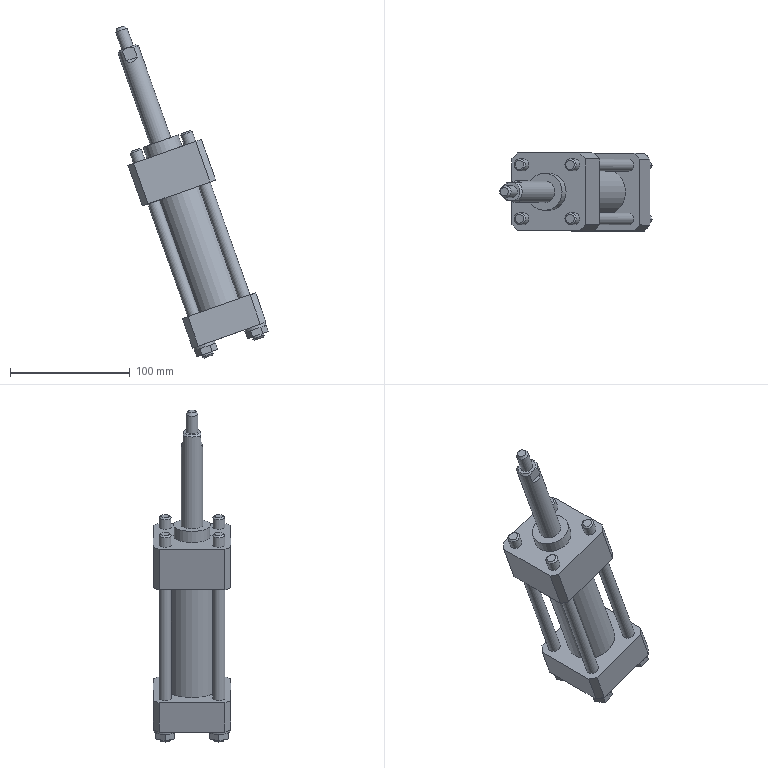Part | STEP file | HYDRAULIC-CYLINDER-1_id470_x_t | 1 solid | 118 faces | box 127.502 x 65 x 277.497 mm | volume 457053 mm3 | plane 87 | cylinder 20 | cone 11 | commonest cylinder face diameters 10 x13 18.4 x4 18 x1 31 x1 40 x1